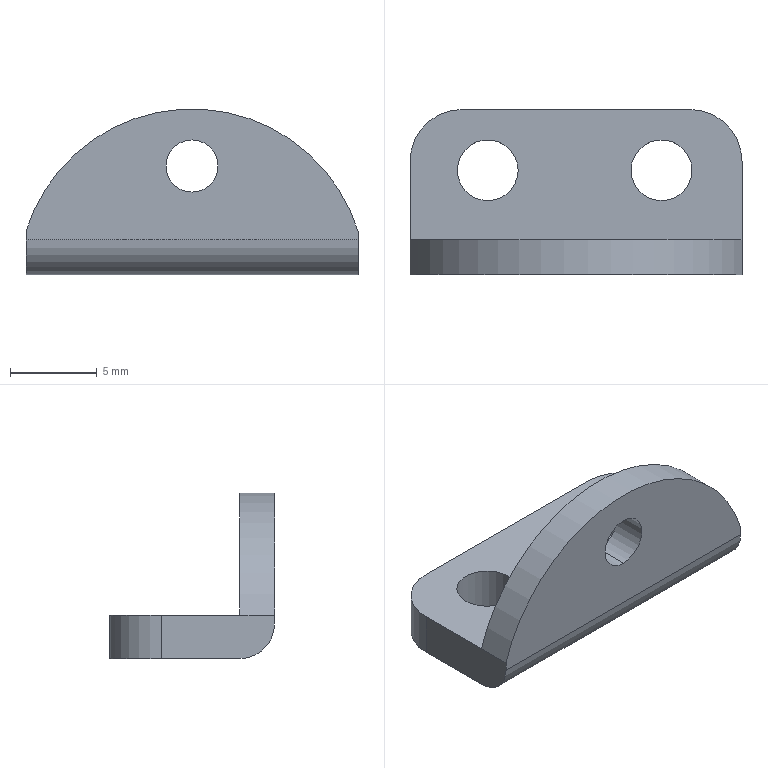Part | SolidWorks | features Extrusion 1, Fillet 1, ICE 1 | 1 solid | 17 faces | box 19.1 x 9.5 x 9.534 mm | volume 562.61 mm3 | cylinder 10 | plane 7 | commonest cylinder face diameters 3.5 x4 3 x2 6 x2 4 x1 20 x1
STEP:
#1=CARTESIAN_POINT('',(0.,-2.75,7.75));
#2=VERTEX_POINT('',#1);
#3=CARTESIAN_POINT('',(0.,-2.75,4.75));
#4=VERTEX_POINT('',#3);
#5=CARTESIAN_POINT('',(0.,-2.75,6.25));
#6=DIRECTION('',(0.,-1.,0.));
#7=DIRECTION('',(0.,0.,-1.));
#8=AXIS2_PLACEMENT_3D('',#5,#6,#7);
#9=CIRCLE('',#8,1.5);
#10=EDGE_CURVE('',#2,#4,#9,.T.);
#11=ORIENTED_EDGE('',*,*,#10,.F.);
#12=CARTESIAN_POINT('',(0.,-4.75,7.75));
#13=VERTEX_POINT('',#12);
#14=CARTESIAN_POINT('',(0.,-2.75,7.75));
#15=DIRECTION('',(0.,-1.,0.));
#16=VECTOR('',#15,1000.);
#17=LINE('',#14,#16);
#18=EDGE_CURVE('',#2,#13,#17,.T.);
#19=ORIENTED_EDGE('',*,*,#18,.T.);
#20=CARTESIAN_POINT('',(0.,-4.75,4.75));
#21=VERTEX_POINT('',#20);
#22=CARTESIAN_POINT('',(0.,-4.75,6.25));
#23=DIRECTION('',(0.,-1.,0.));
#24=DIRECTION('',(0.,0.,-1.));
#25=AXIS2_PLACEMENT_3D('',#22,#23,#24);
#26=CIRCLE('',#25,1.5);
#27=EDGE_CURVE('',#13,#21,#26,.T.);
#28=ORIENTED_EDGE('',*,*,#27,.T.);
#29=CARTESIAN_POINT('',(0.,-2.75,4.75));
#30=DIRECTION('',(0.,-1.,0.));
#31=VECTOR('',#30,1000.);
#32=LINE('',#29,#31);
#33=EDGE_CURVE('',#4,#21,#32,.T.);
#34=ORIENTED_EDGE('',*,*,#33,.F.);
#35=EDGE_LOOP('',(#11,#19,#28,#34));
#36=FACE_OUTER_BOUND('',#35,.T.);
#37=CARTESIAN_POINT('',(0.,-2.75,6.25));
#38=DIRECTION('',(0.,-1.,0.));
#39=DIRECTION('',(0.,0.,-1.));
#40=AXIS2_PLACEMENT_3D('',#37,#38,#39);
#41=CYLINDRICAL_SURFACE('',#40,1.5);
#42=ADVANCED_FACE('',(#36),#41,.F.);
#43=CARTESIAN_POINT('',(-6.829,1.25,2.5));
#44=VERTEX_POINT('',#43);
#45=CARTESIAN_POINT('',(-3.329,1.25,2.5));
#46=VERTEX_POINT('',#45);
#47=CARTESIAN_POINT('',(-5.079,1.25,2.5));
#48=DIRECTION('',(0.,0.,1.));
#49=DIRECTION('',(1.,0.,0.));
#50=AXIS2_PLACEMENT_3D('',#47,#48,#49);
#51=CIRCLE('',#50,1.75);
#52=EDGE_CURVE('',#44,#46,#51,.T.);
#53=ORIENTED_EDGE('',*,*,#52,.T.);
#54=CARTESIAN_POINT('',(-3.329,1.25,0.));
#55=VERTEX_POINT('',#54);
#56=CARTESIAN_POINT('',(-3.329,1.25,2.5));
#57=DIRECTION('',(0.,0.,-1.));
#58=VECTOR('',#57,1000.);
#59=LINE('',#56,#58);
#60=EDGE_CURVE('',#46,#55,#59,.T.);
#61=ORIENTED_EDGE('',*,*,#60,.T.);
#62=CARTESIAN_POINT('',(-6.829,1.25,0.));
#63=VERTEX_POINT('',#62);
#64=CARTESIAN_POINT('',(-5.079,1.25,0.));
#65=DIRECTION('',(0.,0.,1.));
#66=DIRECTION('',(1.,0.,0.));
#67=AXIS2_PLACEMENT_3D('',#64,#65,#66);
#68=CIRCLE('',#67,1.75);
#69=EDGE_CURVE('',#63,#55,#68,.T.);
#70=ORIENTED_EDGE('',*,*,#69,.F.);
#71=CARTESIAN_POINT('',(-6.829,1.25,2.5));
#72=DIRECTION('',(0.,0.,-1.));
#73=VECTOR('',#72,1000.);
#74=LINE('',#71,#73);
#75=EDGE_CURVE('',#44,#63,#74,.T.);
#76=ORIENTED_EDGE('',*,*,#75,.F.);
#77=EDGE_LOOP('',(#53,#61,#70,#76));
#78=FACE_OUTER_BOUND('',#77,.T.);
#79=CARTESIAN_POINT('',(-5.079,1.25,2.5));
#80=DIRECTION('',(0.,0.,-1.));
#81=DIRECTION('',(-1.,0.,0.));
#82=AXIS2_PLACEMENT_3D('',#79,#80,#81);
#83=CYLINDRICAL_SURFACE('',#82,1.75);
#84=ADVANCED_FACE('',(#78),#83,.F.);
#85=CARTESIAN_POINT('',(3.171,1.25,2.5));
#86=VERTEX_POINT('',#85);
#87=CARTESIAN_POINT('',(6.671,1.25,2.5));
#88=VERTEX_POINT('',#87);
#89=CARTESIAN_POINT('',(4.921,1.25,2.5));
#90=DIRECTION('',(0.,0.,1.));
#91=DIRECTION('',(1.,0.,0.));
#92=AXIS2_PLACEMENT_3D('',#89,#90,#91);
#93=CIRCLE('',#92,1.75);
#94=EDGE_CURVE('',#86,#88,#93,.T.);
#95=ORIENTED_EDGE('',*,*,#94,.T.);
#96=CARTESIAN_POINT('',(6.671,1.25,0.));
#97=VERTEX_POINT('',#96);
#98=CARTESIAN_POINT('',(6.671,1.25,2.5));
#99=DIRECTION('',(0.,0.,-1.));
#100=VECTOR('',#99,1000.);
#101=LINE('',#98,#100);
#102=EDGE_CURVE('',#88,#97,#101,.T.);
#103=ORIENTED_EDGE('',*,*,#102,.T.);
#104=CARTESIAN_POINT('',(3.171,1.25,0.));
#105=VERTEX_POINT('',#104);
#106=CARTESIAN_POINT('',(4.921,1.25,0.));
#107=DIRECTION('',(0.,0.,1.));
#108=DIRECTION('',(1.,0.,0.));
#109=AXIS2_PLACEMENT_3D('',#106,#107,#108);
#110=CIRCLE('',#109,1.75);
#111=EDGE_CURVE('',#105,#97,#110,.T.);
#112=ORIENTED_EDGE('',*,*,#111,.F.);
#113=CARTESIAN_POINT('',(3.171,1.25,2.5));
#114=DIRECTION('',(0.,0.,-1.));
#115=VECTOR('',#114,1000.);
#116=LINE('',#113,#115);
#117=EDGE_CURVE('',#86,#105,#116,.T.);
#118=ORIENTED_EDGE('',*,*,#117,.F.);
#119=EDGE_LOOP('',(#95,#103,#112,#118));
#120=FACE_OUTER_BOUND('',#119,.T.);
#121=CARTESIAN_POINT('',(4.921,1.25,2.5));
#122=DIRECTION('',(0.,0.,-1.));
#123=DIRECTION('',(-1.,0.,0.));
#124=AXIS2_PLACEMENT_3D('',#121,#122,#123);
#125=CYLINDRICAL_SURFACE('',#124,1.75);
#126=ADVANCED_FACE('',(#120),#125,.F.);
#127=ORIENTED_EDGE('',*,*,#52,.F.);
#128=CARTESIAN_POINT('',(-5.079,1.25,2.5));
#129=DIRECTION('',(0.,0.,1.));
#130=DIRECTION('',(1.,0.,0.));
#131=AXIS2_PLACEMENT_3D('',#128,#129,#130);
#132=CIRCLE('',#131,1.75);
#133=EDGE_CURVE('',#46,#44,#132,.T.);
#134=ORIENTED_EDGE('',*,*,#133,.F.);
#135=EDGE_LOOP('',(#127,#134));
#136=FACE_BOUND('',#135,.T.);
#137=ORIENTED_EDGE('',*,*,#94,.F.);
#138=CARTESIAN_POINT('',(4.921,1.25,2.5));
#139=DIRECTION('',(0.,0.,1.));
#140=DIRECTION('',(1.,0.,0.));
#141=AXIS2_PLACEMENT_3D('',#138,#139,#140);
#142=CIRCLE('',#141,1.75);
#143=EDGE_CURVE('',#88,#86,#142,.T.);
#144=ORIENTED_EDGE('',*,*,#143,.F.);
#145=EDGE_LOOP('',(#137,#144));
#146=FACE_BOUND('',#145,.T.);
#147=CARTESIAN_POINT('',(-9.55,-2.75,2.5));
#148=VERTEX_POINT('',#147);
#149=CARTESIAN_POINT('',(9.55,-2.75,2.5));
#150=VERTEX_POINT('',#149);
#151=CARTESIAN_POINT('',(-9.55,-2.75,2.5));
#152=DIRECTION('',(1.,0.,0.));
#153=VECTOR('',#152,1000.);
#154=LINE('',#151,#153);
#155=EDGE_CURVE('',#148,#150,#154,.T.);
#156=ORIENTED_EDGE('',*,*,#155,.T.);
#157=CARTESIAN_POINT('',(9.55,1.75,2.5));
#158=VERTEX_POINT('',#157);
#159=CARTESIAN_POINT('',(9.55,-4.75,2.5));
#160=DIRECTION('',(0.,1.,0.));
#161=VECTOR('',#160,1000.);
#162=LINE('',#159,#161);
#163=EDGE_CURVE('',#150,#158,#162,.T.);
#164=ORIENTED_EDGE('',*,*,#163,.T.);
#165=CARTESIAN_POINT('',(6.55,4.75,2.5));
#166=VERTEX_POINT('',#165);
#167=CARTESIAN_POINT('',(6.55,1.75,2.5));
#168=DIRECTION('',(0.,0.,1.));
#169=DIRECTION('',(-1.,0.,0.));
#170=AXIS2_PLACEMENT_3D('',#167,#168,#169);
#171=CIRCLE('',#170,3.);
#172=EDGE_CURVE('',#158,#166,#171,.T.);
#173=ORIENTED_EDGE('',*,*,#172,.T.);
#174=CARTESIAN_POINT('',(-6.55,4.75,2.5));
#175=VERTEX_POINT('',#174);
#176=CARTESIAN_POINT('',(-6.55,4.75,2.5));
#177=DIRECTION('',(-1.,0.,0.));
#178=VECTOR('',#177,1000.);
#179=LINE('',#176,#178);
#180=EDGE_CURVE('',#166,#175,#179,.T.);
#181=ORIENTED_EDGE('',*,*,#180,.T.);
#182=CARTESIAN_POINT('',(-9.55,1.75,2.5));
#183=VERTEX_POINT('',#182);
#184=CARTESIAN_POINT('',(-6.55,1.75,2.5));
#185=DIRECTION('',(0.,0.,1.));
#186=DIRECTION('',(-1.,0.,0.));
#187=AXIS2_PLACEMENT_3D('',#184,#185,#186);
#188=CIRCLE('',#187,3.);
#189=EDGE_CURVE('',#175,#183,#188,.T.);
#190=ORIENTED_EDGE('',*,*,#189,.T.);
#191=CARTESIAN_POINT('',(-9.55,-4.75,2.5));
#192=DIRECTION('',(0.,-1.,0.));
#193=VECTOR('',#192,1000.);
#194=LINE('',#191,#193);
#195=EDGE_CURVE('',#183,#148,#194,.T.);
#196=ORIENTED_EDGE('',*,*,#195,.T.);
#197=EDGE_LOOP('',(#156,#164,#173,#181,#190,#196));
#198=FACE_OUTER_BOUND('',#197,.T.);
#199=CARTESIAN_POINT('',(-6.55,1.75,2.5));
#200=DIRECTION('',(0.,0.,-1.));
#201=DIRECTION('',(-1.,0.,0.));
#202=AXIS2_PLACEMENT_3D('',#199,#200,#201);
#203=PLANE('',#202);
#204=ADVANCED_FACE('',(#136,#146,#198),#203,.F.);
#205=ORIENTED_EDGE('',*,*,#111,.T.);
#206=CARTESIAN_POINT('',(4.921,1.25,0.));
#207=DIRECTION('',(0.,0.,1.));
#208=DIRECTION('',(1.,0.,0.));
#209=AXIS2_PLACEMENT_3D('',#206,#207,#208);
#210=CIRCLE('',#209,1.75);
#211=EDGE_CURVE('',#97,#105,#210,.T.);
#212=ORIENTED_EDGE('',*,*,#211,.T.);
#213=EDGE_LOOP('',(#205,#212));
#214=FACE_BOUND('',#213,.T.);
#215=CARTESIAN_POINT('',(9.55,-2.75,0.));
#216=VERTEX_POINT('',#215);
#217=CARTESIAN_POINT('',(9.55,1.75,0.));
#218=VERTEX_POINT('',#217);
#219=CARTESIAN_POINT('',(9.55,-4.75,0.));
#220=DIRECTION('',(0.,1.,0.));
#221=VECTOR('',#220,1000.);
#222=LINE('',#219,#221);
#223=EDGE_CURVE('',#216,#218,#222,.T.);
#224=ORIENTED_EDGE('',*,*,#223,.F.);
#225=CARTESIAN_POINT('',(-9.55,-2.75,0.));
#226=VERTEX_POINT('',#225);
#227=CARTESIAN_POINT('',(-9.55,-2.75,0.));
#228=DIRECTION('',(-1.,0.,0.));
#229=VECTOR('',#228,1000.);
#230=LINE('',#227,#229);
#231=EDGE_CURVE('',#216,#226,#230,.T.);
#232=ORIENTED_EDGE('',*,*,#231,.T.);
#233=CARTESIAN_POINT('',(-9.55,1.75,0.));
#234=VERTEX_POINT('',#233);
#235=CARTESIAN_POINT('',(-9.55,-4.75,0.));
#236=DIRECTION('',(0.,-1.,0.));
#237=VECTOR('',#236,1000.);
#238=LINE('',#235,#237);
#239=EDGE_CURVE('',#234,#226,#238,.T.);
#240=ORIENTED_EDGE('',*,*,#239,.F.);
#241=CARTESIAN_POINT('',(-6.55,4.75,0.));
#242=VERTEX_POINT('',#241);
#243=CARTESIAN_POINT('',(-6.55,1.75,0.));
#244=DIRECTION('',(0.,0.,1.));
#245=DIRECTION('',(-1.,0.,0.));
#246=AXIS2_PLACEMENT_3D('',#243,#244,#245);
#247=CIRCLE('',#246,3.);
#248=EDGE_CURVE('',#242,#234,#247,.T.);
#249=ORIENTED_EDGE('',*,*,#248,.F.);
#250=CARTESIAN_POINT('',(6.55,4.75,0.));
#251=VERTEX_POINT('',#250);
#252=CARTESIAN_POINT('',(-6.55,4.75,0.));
#253=DIRECTION('',(-1.,0.,0.));
#254=VECTOR('',#253,1000.);
#255=LINE('',#252,#254);
#256=EDGE_CURVE('',#251,#242,#255,.T.);
#257=ORIENTED_EDGE('',*,*,#256,.F.);
#258=CARTESIAN_POINT('',(6.55,1.75,0.));
#259=DIRECTION('',(0.,0.,1.));
#260=DIRECTION('',(-1.,0.,0.));
#261=AXIS2_PLACEMENT_3D('',#258,#259,#260);
#262=CIRCLE('',#261,3.);
#263=EDGE_CURVE('',#218,#251,#262,.T.);
#264=ORIENTED_EDGE('',*,*,#263,.F.);
#265=EDGE_LOOP('',(#224,#232,#240,#249,#257,#264));
#266=FACE_OUTER_BOUND('',#265,.T.);
#267=ORIENTED_EDGE('',*,*,#69,.T.);
#268=CARTESIAN_POINT('',(-5.079,1.25,0.));
#269=DIRECTION('',(0.,0.,1.));
#270=DIRECTION('',(1.,0.,0.));
#271=AXIS2_PLACEMENT_3D('',#268,#269,#270);
#272=CIRCLE('',#271,1.75);
#273=EDGE_CURVE('',#55,#63,#272,.T.);
#274=ORIENTED_EDGE('',*,*,#273,.T.);
#275=EDGE_LOOP('',(#267,#274));
#276=FACE_BOUND('',#275,.T.);
#277=CARTESIAN_POINT('',(-6.55,1.75,0.));
#278=DIRECTION('',(0.,0.,-1.));
#279=DIRECTION('',(-1.,0.,0.));
#280=AXIS2_PLACEMENT_3D('',#277,#278,#279);
#281=PLANE('',#280);
#282=ADVANCED_FACE('',(#214,#266,#276),#281,.T.);
#283=ORIENTED_EDGE('',*,*,#239,.T.);
#284=CARTESIAN_POINT('',(-9.55,-4.75,2.));
#285=VERTEX_POINT('',#284);
#286=CARTESIAN_POINT('',(-9.55,-2.75,2.));
#287=DIRECTION('',(-1.,0.,0.));
#288=DIRECTION('',(0.,0.,-1.));
#289=AXIS2_PLACEMENT_3D('',#286,#287,#288);
#290=CIRCLE('',#289,2.);
#291=EDGE_CURVE('',#226,#285,#290,.T.);
#292=ORIENTED_EDGE('',*,*,#291,.T.);
#293=CARTESIAN_POINT('',(-9.55,-4.75,2.5));
#294=VERTEX_POINT('',#293);
#295=CARTESIAN_POINT('',(-9.55,-4.75,2.5));
#296=DIRECTION('',(0.,0.,-1.));
#297=VECTOR('',#296,1000.);
#298=LINE('',#295,#297);
#299=EDGE_CURVE('',#294,#285,#298,.T.);
#300=ORIENTED_EDGE('',*,*,#299,.F.);
#301=CARTESIAN_POINT('',(-9.55,-2.75,2.5));
#302=DIRECTION('',(0.,-1.,0.));
#303=VECTOR('',#302,1000.);
#304=LINE('',#301,#303);
#305=EDGE_CURVE('',#148,#294,#304,.T.);
#306=ORIENTED_EDGE('',*,*,#305,.F.);
#307=ORIENTED_EDGE('',*,*,#195,.F.);
#308=CARTESIAN_POINT('',(-9.55,1.75,2.5));
#309=DIRECTION('',(0.,0.,-1.));
#310=VECTOR('',#309,1000.);
#311=LINE('',#308,#310);
#312=EDGE_CURVE('',#183,#234,#311,.T.);
#313=ORIENTED_EDGE('',*,*,#312,.T.);
#314=EDGE_LOOP('',(#283,#292,#300,#306,#307,#313));
#315=FACE_OUTER_BOUND('',#314,.T.);
#316=CARTESIAN_POINT('',(-9.55,-4.75,2.5));
#317=DIRECTION('',(1.,0.,0.));
#318=DIRECTION('',(0.,0.,-1.));
#319=AXIS2_PLACEMENT_3D('',#316,#317,#318);
#320=PLANE('',#319);
#321=ADVANCED_FACE('',(#315),#320,.F.);
#322=ORIENTED_EDGE('',*,*,#299,.T.);
#323=CARTESIAN_POINT('',(9.55,-4.75,2.));
#324=VERTEX_POINT('',#323);
#325=CARTESIAN_POINT('',(9.55,-4.75,2.));
#326=DIRECTION('',(1.,0.,0.));
#327=VECTOR('',#326,1000.);
#328=LINE('',#325,#327);
#329=EDGE_CURVE('',#285,#324,#328,.T.);
#330=ORIENTED_EDGE('',*,*,#329,.T.);
#331=CARTESIAN_POINT('',(9.55,-4.75,2.5));
#332=VERTEX_POINT('',#331);
#333=CARTESIAN_POINT('',(9.55,-4.75,2.5));
#334=DIRECTION('',(0.,0.,-1.));
#335=VECTOR('',#334,1000.);
#336=LINE('',#333,#335);
#337=EDGE_CURVE('',#332,#324,#336,.T.);
#338=ORIENTED_EDGE('',*,*,#337,.F.);
#339=CARTESIAN_POINT('',(0.,-4.75,-0.4661));
#340=DIRECTION('',(0.,-1.,0.));
#341=DIRECTION('',(0.,0.,-1.));
#342=AXIS2_PLACEMENT_3D('',#339,#340,#341);
#343=CIRCLE('',#342,10.);
#344=EDGE_CURVE('',#332,#294,#343,.T.);
#345=ORIENTED_EDGE('',*,*,#344,.T.);
#346=EDGE_LOOP('',(#322,#330,#338,#345));
#347=FACE_OUTER_BOUND('',#346,.T.);
#348=CARTESIAN_POINT('',(0.,-4.75,6.25));
#349=DIRECTION('',(0.,-1.,0.));
#350=DIRECTION('',(0.,0.,-1.));
#351=AXIS2_PLACEMENT_3D('',#348,#349,#350);
#352=CIRCLE('',#351,1.5);
#353=EDGE_CURVE('',#21,#13,#352,.T.);
#354=ORIENTED_EDGE('',*,*,#353,.F.);
#355=ORIENTED_EDGE('',*,*,#27,.F.);
#356=EDGE_LOOP('',(#354,#355));
#357=FACE_BOUND('',#356,.T.);
#358=CARTESIAN_POINT('',(-9.55,-4.75,2.5));
#359=DIRECTION('',(0.,1.,0.));
#360=DIRECTION('',(0.,0.,1.));
#361=AXIS2_PLACEMENT_3D('',#358,#359,#360);
#362=PLANE('',#361);
#363=ADVANCED_FACE('',(#347,#357),#362,.F.);
#364=ORIENTED_EDGE('',*,*,#337,.T.);
#365=CARTESIAN_POINT('',(9.55,-2.75,2.));
#366=DIRECTION('',(1.,0.,0.));
#367=DIRECTION('',(0.,0.,1.));
#368=AXIS2_PLACEMENT_3D('',#365,#366,#367);
#369=CIRCLE('',#368,2.);
#370=EDGE_CURVE('',#324,#216,#369,.T.);
#371=ORIENTED_EDGE('',*,*,#370,.T.);
#372=ORIENTED_EDGE('',*,*,#223,.T.);
#373=CARTESIAN_POINT('',(9.55,1.75,2.5));
#374=DIRECTION('',(0.,0.,-1.));
#375=VECTOR('',#374,1000.);
#376=LINE('',#373,#375);
#377=EDGE_CURVE('',#158,#218,#376,.T.);
#378=ORIENTED_EDGE('',*,*,#377,.F.);
#379=ORIENTED_EDGE('',*,*,#163,.F.);
#380=CARTESIAN_POINT('',(9.55,-4.75,2.5));
#381=DIRECTION('',(0.,1.,0.));
#382=VECTOR('',#381,1000.);
#383=LINE('',#380,#382);
#384=EDGE_CURVE('',#332,#150,#383,.T.);
#385=ORIENTED_EDGE('',*,*,#384,.F.);
#386=EDGE_LOOP('',(#364,#371,#372,#378,#379,#385));
#387=FACE_OUTER_BOUND('',#386,.T.);
#388=CARTESIAN_POINT('',(9.55,-4.75,2.5));
#389=DIRECTION('',(-1.,0.,0.));
#390=DIRECTION('',(0.,0.,1.));
#391=AXIS2_PLACEMENT_3D('',#388,#389,#390);
#392=PLANE('',#391);
#393=ADVANCED_FACE('',(#387),#392,.F.);
#394=ORIENTED_EDGE('',*,*,#263,.T.);
#395=CARTESIAN_POINT('',(6.55,4.75,2.5));
#396=DIRECTION('',(0.,0.,-1.));
#397=VECTOR('',#396,1000.);
#398=LINE('',#395,#397);
#399=EDGE_CURVE('',#166,#251,#398,.T.);
#400=ORIENTED_EDGE('',*,*,#399,.F.);
#401=ORIENTED_EDGE('',*,*,#172,.F.);
#402=ORIENTED_EDGE('',*,*,#377,.T.);
#403=EDGE_LOOP('',(#394,#400,#401,#402));
#404=FACE_OUTER_BOUND('',#403,.T.);
#405=CARTESIAN_POINT('',(6.55,1.75,2.5));
#406=DIRECTION('',(0.,0.,-1.));
#407=DIRECTION('',(-1.,0.,0.));
#408=AXIS2_PLACEMENT_3D('',#405,#406,#407);
#409=CYLINDRICAL_SURFACE('',#408,3.);
#410=ADVANCED_FACE('',(#404),#409,.T.);
#411=ORIENTED_EDGE('',*,*,#256,.T.);
#412=CARTESIAN_POINT('',(-6.55,4.75,2.5));
#413=DIRECTION('',(0.,0.,-1.));
#414=VECTOR('',#413,1000.);
#415=LINE('',#412,#414);
#416=EDGE_CURVE('',#175,#242,#415,.T.);
#417=ORIENTED_EDGE('',*,*,#416,.F.);
#418=ORIENTED_EDGE('',*,*,#180,.F.);
#419=ORIENTED_EDGE('',*,*,#399,.T.);
#420=EDGE_LOOP('',(#411,#417,#418,#419));
#421=FACE_OUTER_BOUND('',#420,.T.);
#422=CARTESIAN_POINT('',(-6.55,4.75,2.5));
#423=DIRECTION('',(0.,-1.,0.));
#424=DIRECTION('',(0.,0.,-1.));
#425=AXIS2_PLACEMENT_3D('',#422,#423,#424);
#426=PLANE('',#425);
#427=ADVANCED_FACE('',(#421),#426,.F.);
#428=ORIENTED_EDGE('',*,*,#248,.T.);
#429=ORIENTED_EDGE('',*,*,#312,.F.);
#430=ORIENTED_EDGE('',*,*,#189,.F.);
#431=ORIENTED_EDGE('',*,*,#416,.T.);
#432=EDGE_LOOP('',(#428,#429,#430,#431));
#433=FACE_OUTER_BOUND('',#432,.T.);
#434=CARTESIAN_POINT('',(-6.55,1.75,2.5));
#435=DIRECTION('',(0.,0.,-1.));
#436=DIRECTION('',(-1.,0.,0.));
#437=AXIS2_PLACEMENT_3D('',#434,#435,#436);
#438=CYLINDRICAL_SURFACE('',#437,3.);
#439=ADVANCED_FACE('',(#433),#438,.T.);
#440=ORIENTED_EDGE('',*,*,#102,.F.);
#441=ORIENTED_EDGE('',*,*,#143,.T.);
#442=ORIENTED_EDGE('',*,*,#117,.T.);
#443=ORIENTED_EDGE('',*,*,#211,.F.);
#444=EDGE_LOOP('',(#440,#441,#442,#443));
#445=FACE_OUTER_BOUND('',#444,.T.);
#446=CARTESIAN_POINT('',(4.921,1.25,2.5));
#447=DIRECTION('',(0.,0.,-1.));
#448=DIRECTION('',(-1.,0.,0.));
#449=AXIS2_PLACEMENT_3D('',#446,#447,#448);
#450=CYLINDRICAL_SURFACE('',#449,1.75);
#451=ADVANCED_FACE('',(#445),#450,.F.);
#452=ORIENTED_EDGE('',*,*,#60,.F.);
#453=ORIENTED_EDGE('',*,*,#133,.T.);
#454=ORIENTED_EDGE('',*,*,#75,.T.);
#455=ORIENTED_EDGE('',*,*,#273,.F.);
#456=EDGE_LOOP('',(#452,#453,#454,#455));
#457=FACE_OUTER_BOUND('',#456,.T.);
#458=CARTESIAN_POINT('',(-5.079,1.25,2.5));
#459=DIRECTION('',(0.,0.,-1.));
#460=DIRECTION('',(-1.,0.,0.));
#461=AXIS2_PLACEMENT_3D('',#458,#459,#460);
#462=CYLINDRICAL_SURFACE('',#461,1.75);
#463=ADVANCED_FACE('',(#457),#462,.F.);
#464=ORIENTED_EDGE('',*,*,#344,.F.);
#465=ORIENTED_EDGE('',*,*,#384,.T.);
#466=CARTESIAN_POINT('',(0.,-2.75,-0.4661));
#467=DIRECTION('',(0.,-1.,0.));
#468=DIRECTION('',(0.,0.,-1.));
#469=AXIS2_PLACEMENT_3D('',#466,#467,#468);
#470=CIRCLE('',#469,10.);
#471=EDGE_CURVE('',#150,#148,#470,.T.);
#472=ORIENTED_EDGE('',*,*,#471,.T.);
#473=ORIENTED_EDGE('',*,*,#305,.T.);
#474=EDGE_LOOP('',(#464,#465,#472,#473));
#475=FACE_OUTER_BOUND('',#474,.T.);
#476=CARTESIAN_POINT('',(0.,-2.75,-0.4661));
#477=DIRECTION('',(0.,-1.,0.));
#478=DIRECTION('',(0.,0.,-1.));
#479=AXIS2_PLACEMENT_3D('',#476,#477,#478);
#480=CYLINDRICAL_SURFACE('',#479,10.);
#481=ADVANCED_FACE('',(#475),#480,.T.);
#482=CARTESIAN_POINT('',(0.,-2.75,6.25));
#483=DIRECTION('',(0.,-1.,0.));
#484=DIRECTION('',(0.,0.,-1.));
#485=AXIS2_PLACEMENT_3D('',#482,#483,#484);
#486=CIRCLE('',#485,1.5);
#487=EDGE_CURVE('',#4,#2,#486,.T.);
#488=ORIENTED_EDGE('',*,*,#487,.T.);
#489=ORIENTED_EDGE('',*,*,#10,.T.);
#490=EDGE_LOOP('',(#488,#489));
#491=FACE_BOUND('',#490,.T.);
#492=ORIENTED_EDGE('',*,*,#471,.F.);
#493=ORIENTED_EDGE('',*,*,#155,.F.);
#494=EDGE_LOOP('',(#492,#493));
#495=FACE_OUTER_BOUND('',#494,.T.);
#496=CARTESIAN_POINT('',(0.,-2.75,-0.4661));
#497=DIRECTION('',(0.,-1.,0.));
#498=DIRECTION('',(0.,0.,-1.));
#499=AXIS2_PLACEMENT_3D('',#496,#497,#498);
#500=PLANE('',#499);
#501=ADVANCED_FACE('',(#491,#495),#500,.F.);
#502=ORIENTED_EDGE('',*,*,#18,.F.);
#503=ORIENTED_EDGE('',*,*,#487,.F.);
#504=ORIENTED_EDGE('',*,*,#33,.T.);
#505=ORIENTED_EDGE('',*,*,#353,.T.);
#506=EDGE_LOOP('',(#502,#503,#504,#505));
#507=FACE_OUTER_BOUND('',#506,.T.);
#508=CARTESIAN_POINT('',(0.,-2.75,6.25));
#509=DIRECTION('',(0.,-1.,0.));
#510=DIRECTION('',(0.,0.,-1.));
#511=AXIS2_PLACEMENT_3D('',#508,#509,#510);
#512=CYLINDRICAL_SURFACE('',#511,1.5);
#513=ADVANCED_FACE('',(#507),#512,.F.);
#514=ORIENTED_EDGE('',*,*,#291,.F.);
#515=ORIENTED_EDGE('',*,*,#231,.F.);
#516=ORIENTED_EDGE('',*,*,#370,.F.);
#517=ORIENTED_EDGE('',*,*,#329,.F.);
#518=EDGE_LOOP('',(#514,#515,#516,#517));
#519=FACE_OUTER_BOUND('',#518,.T.);
#520=CARTESIAN_POINT('',(-9.55,-2.75,2.));
#521=DIRECTION('',(-1.,0.,0.));
#522=DIRECTION('',(0.,0.,1.));
#523=AXIS2_PLACEMENT_3D('',#520,#521,#522);
#524=CYLINDRICAL_SURFACE('',#523,2.);
#525=ADVANCED_FACE('',(#519),#524,.T.);
#526=CLOSED_SHELL('',(#42,#84,#126,#204,#282,#321,#363,#393,#410,#427,#439,#451,#463,#481,#501,#513,#525));
#527=MANIFOLD_SOLID_BREP('',#526);
#528=CARTESIAN_POINT('',(0.,0.,0.));
#529=DIRECTION('',(0.,0.,1.));
#530=DIRECTION('',(1.,0.,0.));
#531=AXIS2_PLACEMENT_3D('',#528,#529,#530);
#532=(LENGTH_UNIT()NAMED_UNIT(*)SI_UNIT(.MILLI.,.METRE.));
#533=UNCERTAINTY_MEASURE_WITH_UNIT(LENGTH_MEASURE(0.00001),#532,'','');
#534=(NAMED_UNIT(*)PLANE_ANGLE_UNIT()SI_UNIT($,.RADIAN.));
#535=(NAMED_UNIT(*)SI_UNIT($,.STERADIAN.)SOLID_ANGLE_UNIT());
#536=(GEOMETRIC_REPRESENTATION_CONTEXT(3)GLOBAL_UNCERTAINTY_ASSIGNED_CONTEXT((#533))GLOBAL_UNIT_ASSIGNED_CONTEXT((#532,#534,#535))REPRESENTATION_CONTEXT('',''));
#537=ADVANCED_BREP_SHAPE_REPRESENTATION('',(#527,#531),#536);